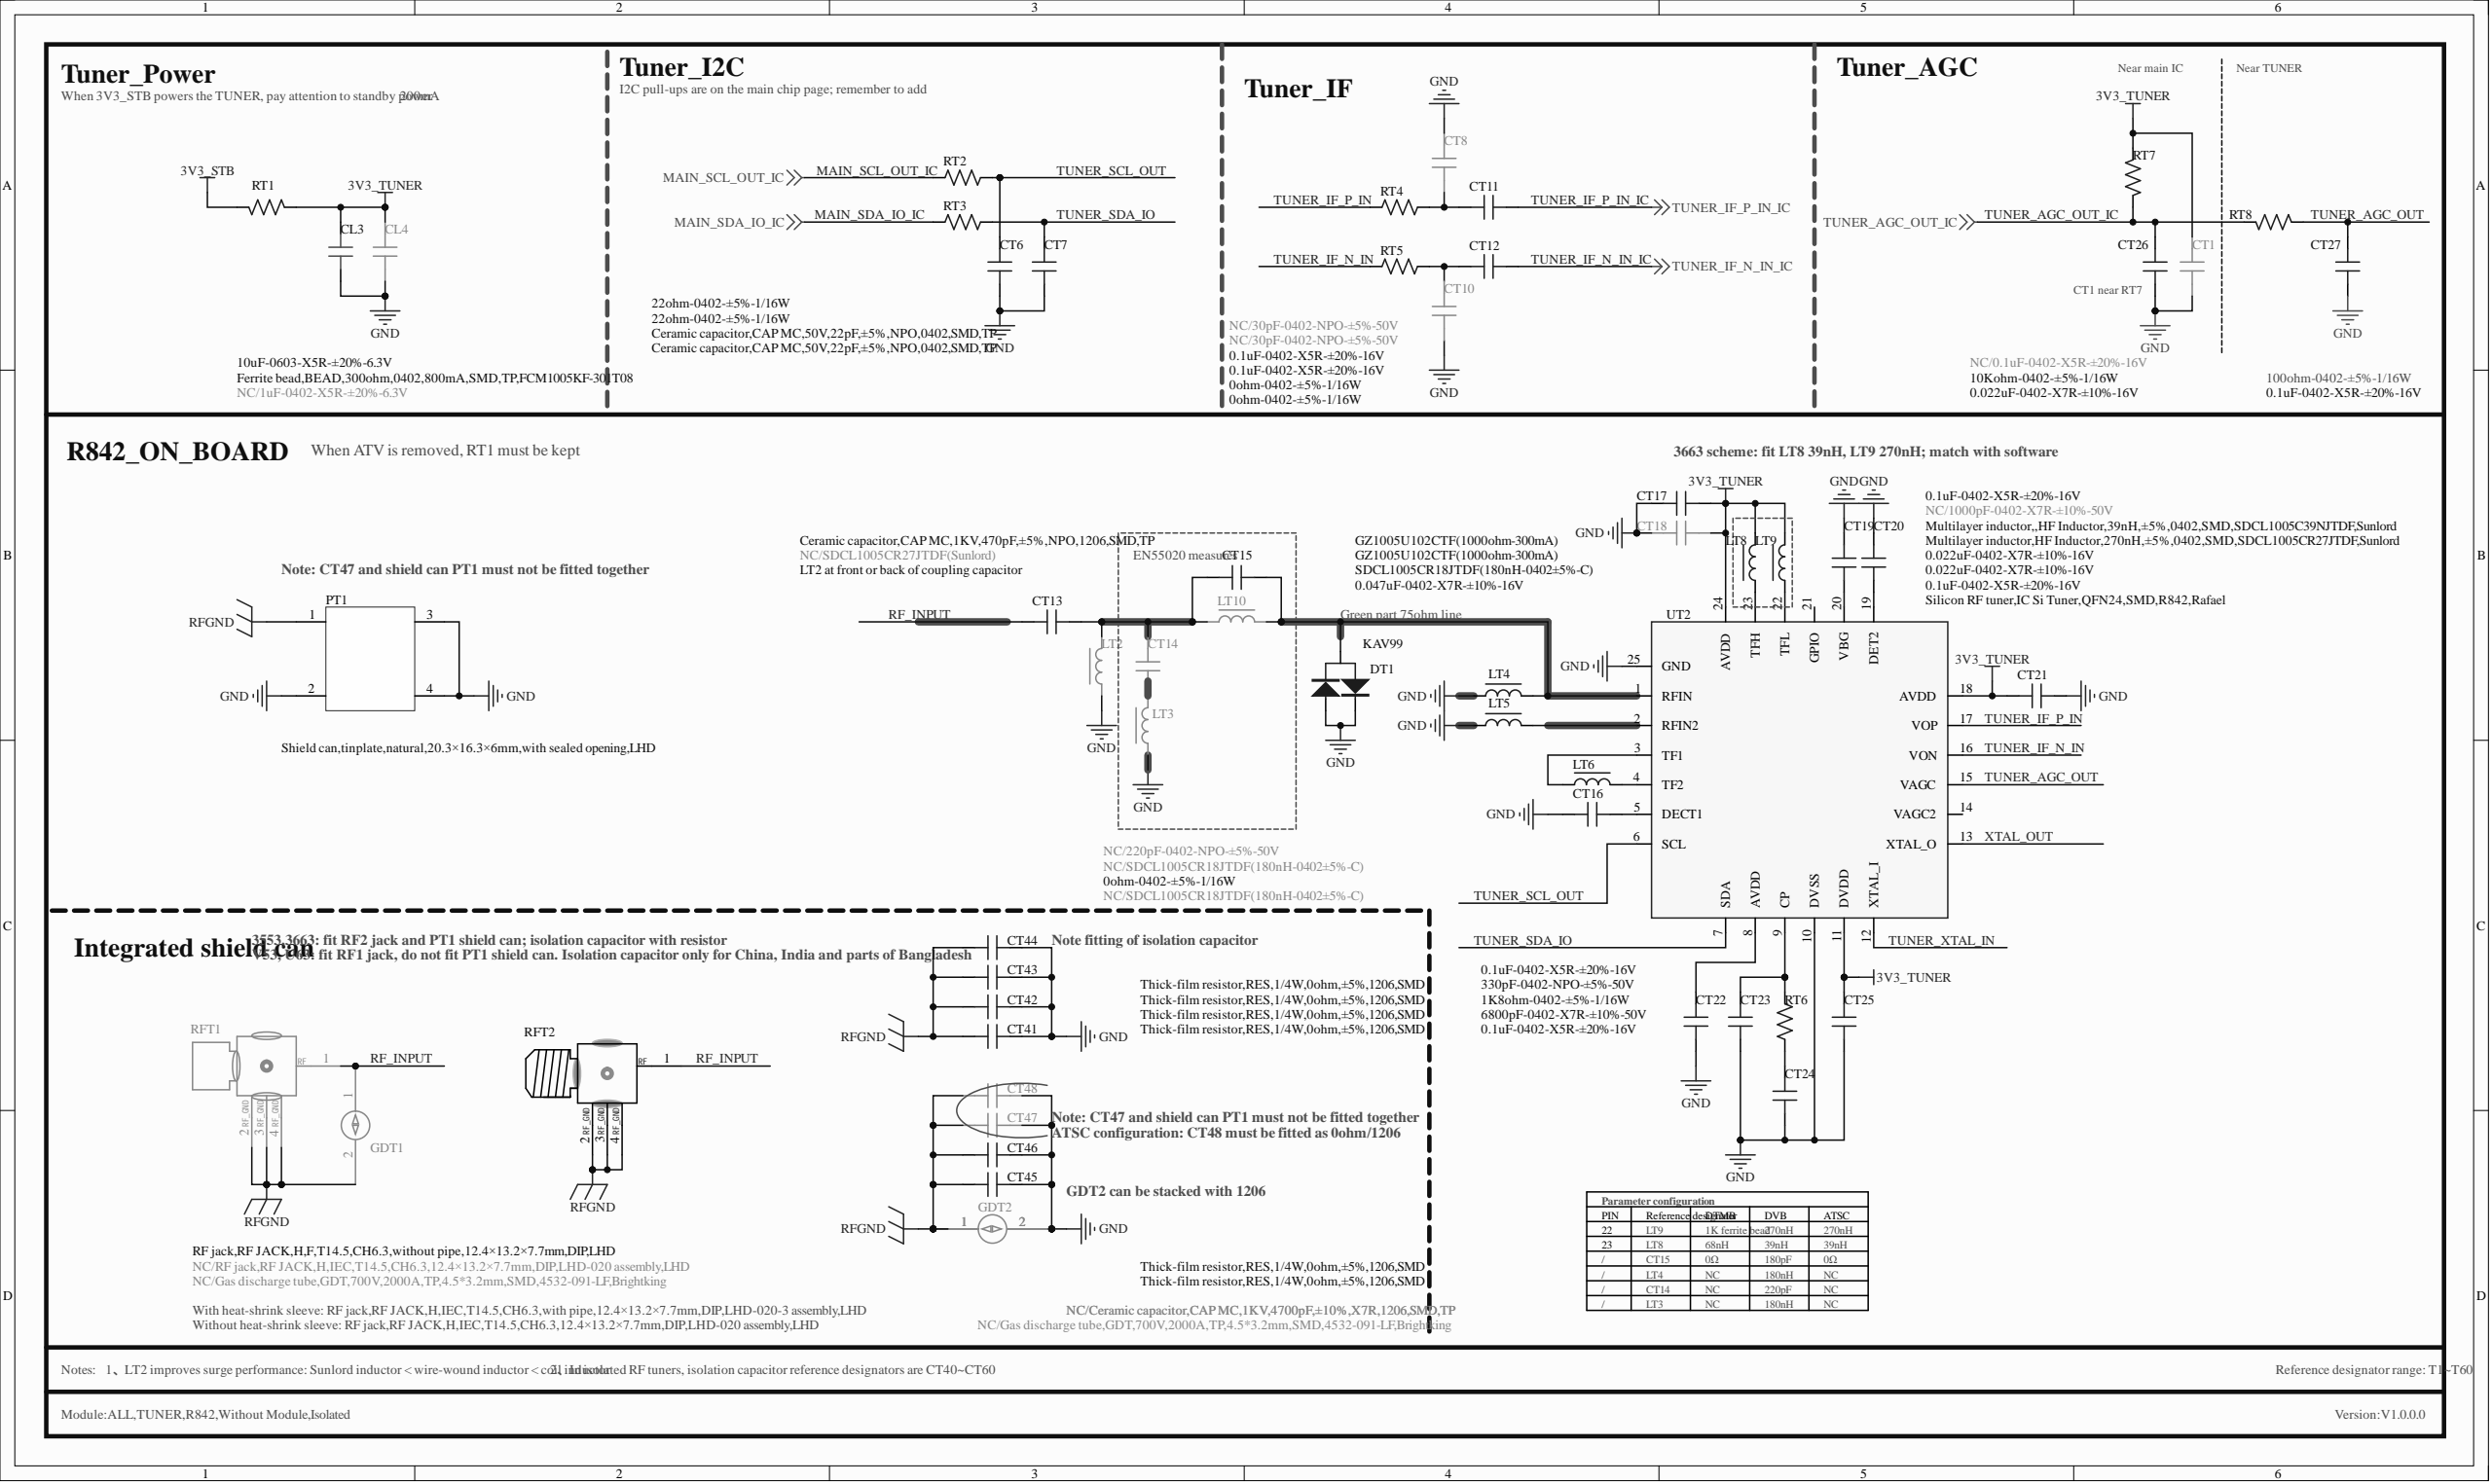Circuit board | Altium Designer | 578 parts | 300 nets | one sheet of the schematic
Parts on this sheet (reference | value | footprint):
CL3 | 10uF-0603-X5R-±20%-6.3V | C0603
CL4 | NC/1uF-0402-X5R-±20%-6.3V | C0402
CT1 | NC/0.1uF-0402-X5R-±20%-16V | C0402
CT6 | Ceramic capacitor,CAP MC,50V,22pF,±5%,NPO,0402,SMD,TP | C0402
CT7 | Ceramic capacitor,CAP MC,50V,22pF,±5%,NPO,0402,SMD,TP | C0402
CT8 | NC/30pF-0402-NPO-±5%-50V | C0402
CT10 | NC/30pF-0402-NPO-±5%-50V | C0402
CT11 | 0.1uF-0402-X5R-±20%-16V | C0402
CT12 | 0.1uF-0402-X5R-±20%-16V | C0402
CT13 | Ceramic capacitor,CAP MC,1KV,470pF,±5%,NPO,1206,SMD,TP | C1206
CT14 | NC/220pF-0402-NPO-±5%-50V | C0402
CT15 | 0ohm-0402-±5%-1/16W | C0402
CT16 | 0.047uF-0402-X7R-±10%-16V | C0402
CT17 | 0.1uF-0402-X5R-±20%-16V | C0402
CT18 | NC/1000pF-0402-X7R-±10%-50V | C0402
CT19 | 0.022uF-0402-X7R-±10%-16V | C0402
CT20 | 0.022uF-0402-X7R-±10%-16V | C0402
CT21 | 0.1uF-0402-X5R-±20%-16V | C0402
CT22 | 0.1uF-0402-X5R-±20%-16V | C0402
CT23 | 330pF-0402-NPO-±5%-50V | C0402
CT24 | 6800pF-0402-X7R-±10%-50V | C0402
CT25 | 0.1uF-0402-X5R-±20%-16V | C0402
CT26 | 0.022uF-0402-X7R-±10%-16V | C0402
CT27 | 0.1uF-0402-X5R-±20%-16V | C0402
CT41 | Thick-film resistor,RES,1/4W,0ohm,±5%,1206,SMD | C1206
CT42 | Thick-film resistor,RES,1/4W,0ohm,±5%,1206,SMD | C1206
CT43 | Thick-film resistor,RES,1/4W,0ohm,±5%,1206,SMD | C1206
CT44 | Thick-film resistor,RES,1/4W,0ohm,±5%,1206,SMD | C1206
CT45 | Thick-film resistor,RES,1/4W,0ohm,±5%,1206,SMD | C1206
CT46 | Thick-film resistor,RES,1/4W,0ohm,±5%,1206,SMD | C1206
CT47 | NC/Ceramic capacitor,CAP MC,1KV,4700pF,±10%,X7R,1206,SMD,TP | C1206
CT48 | NC/Ceramic capacitor,CAP MC,1KV,4700pF,±10%,X7R,1206,SMD,TP | C1206
DT1 | KAV99 | SO-23
GDT1 | NC/Gas discharge tube,GDT,700V,2000A,TP,4.5*3.2mm,SMD,4532-091-LF,Brightking | SMD4532-1
GDT2 | NC/Gas discharge tube,GDT,700V,2000A,TP,4.5*3.2mm,SMD,4532-091-LF,Brightking | SMD4532-1-C1206
LT2 | NC/SDCL1005CR27JTDF(Sunlord) | L0402
LT3 | NC/SDCL1005CR18JTDF(180nH-0402±5%-C) | L0402
LT4 | GZ1005U102CTF(1000ohm-300mA) | L0402
LT5 | GZ1005U102CTF(1000ohm-300mA) | L0402
LT6 | SDCL1005CR18JTDF(180nH-0402±5%-C) | L0402
LT10 | NC/SDCL1005CR18JTDF(180nH-0402±5%-C) | L0402
PT1 | Shield can,tinplate,natural,20.3×16.3×6mm,with sealed opening,LHD | SHIELD(16*20*6)
RFT1 | NC/RF jack,RF JACK,H,IEC,T14.5,CH6.3,12.4×13.2×7.7mm,DIP,LHD-020 assembly,LHD | ANT-IEC14.5-H-4
RFT2 | RF jack,RF JACK,H,F,T14.5,CH6.3,without pipe,12.4×13.2×7.7mm,DIP,LHD | T-13.2×12.4×7.7-F14.5
RT2 | 22ohm-0402-±5%-1/16W | R0402
RT3 | 22ohm-0402-±5%-1/16W | R0402
RT4 | 0ohm-0402-±5%-1/16W | R0402
RT5 | 0ohm-0402-±5%-1/16W | R0402
RT6 | 1K8ohm-0402-±5%-1/16W | R0402
RT7 | 10Kohm-0402-±5%-1/16W | R0402
RT8 | 100ohm-0402-±5%-1/16W | R0402
UT2 | Silicon RF tuner,IC Si Tuner,QFN24,SMD,R842,Rafael | QFN24/0.5-3
Nets of these parts (net: part-pin ...):
XTAL_OUT: UT2-13
TUNER_SDA_IO: CT7-2 RT3-2 UT2-7
TUNER_SCL_OUT: CT6-2 RT2-2 UT2-6
TUNER_IF_P_IN_IC: CT11-1
TUNER_IF_P_IN: RT4-1 UT2-17
TUNER_IF_N_IN_IC: CT12-1
TUNER_IF_N_IN: RT5-1 UT2-16
TUNER_AGC_OUT_IC: CT26-2 RT7-2 RT8-2
TUNER_AGC_OUT: CT27-2 RT8-1 UT2-15
RFGND: CT41-2 CT42-2 CT43-2 CT44-2 CT45-2 CT46-2 CT47-2 CT48-2 GDT1-2 GDT2-1 PT1-1 RFT1-2 RFT1-3 RFT1-4 RFT2-2 RFT2-3 RFT2-4
RF_INPUT: CT13-1 GDT1-1 RFT1-1 RFT2-1
NetLT6_2: LT6-2 UT2-3
NetLT6_1: LT6-1 UT2-4
NetLT5_1: LT5-1 UT2-2
NetCT24_2: CT24-2 RT6-1
NetCT23_2: CT23-2 RT6-2 UT2-9
NetCT22_1: CT22-1 UT2-8
NetCT20_1: CT20-1 UT2-19
NetCT19_2: CT19-2 UT2-20
NetCT16_1: CT16-1 UT2-5
NetCT15_2: CT15-2 DT1-2 LT4-1 LT10-1 UT2-1
NetCT14_2: CT14-2 LT3-1
NetCT13_2: CT13-2 CT14-1 CT15-1 LT2-1 LT10-2
NetCT10_1: CT10-1 CT12-2 RT5-2
NetCT8_2: CT8-2 CT11-2 RT4-2
MAIN_SDA_IO_IC: RT3-1
MAIN_SCL_OUT_IC: RT2-1
GND: CL3-1 CL4-1 CT1-2 CT6-1 CT7-1 CT8-1 CT10-2 CT16-2 CT17-1 CT18-2 CT19-1 CT20-2 CT21-1 CT22-2 CT23-1 CT24-1 CT25-2 CT26-1 CT27-1 CT41-1 CT42-1 CT43-1 CT44-1 CT45-1 CT46-1 CT47-1 CT48-1 DT1-1 DT1-3 GDT2-2 LT2-2 LT3-2 LT4-2 LT5-2 PT1-2 PT1-3 PT1-4 UT2-10 UT2-25
3V3_TUNER: CL3-2 CL4-2 CT1-1 CT17-2 CT18-1 CT21-2 CT25-1 RT7-1 UT2-11 UT2-18 UT2-24